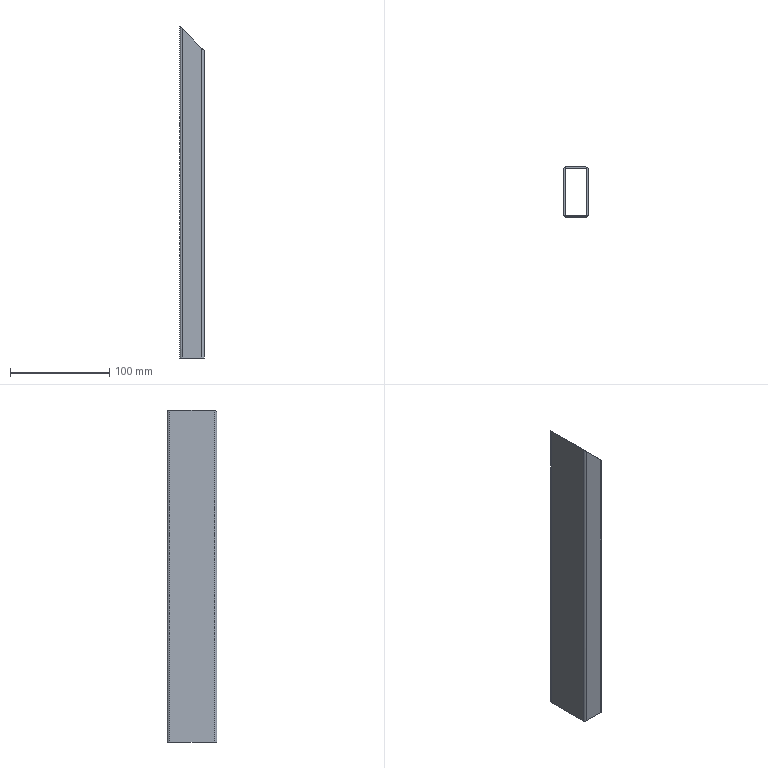Part | STEP file | 6150515 | 1 solid | 18 faces | box 25 x 50 x 334 mm | volume 67995 mm3 | plane 10 | cylinder 8 | commonest cylinder face diameters 2 x4 5 x4
STEP:
#1=CARTESIAN_POINT('',(-12.5,-22.5,0.));
#2=VERTEX_POINT('',#1);
#3=CARTESIAN_POINT('',(-10.,-25.,0.));
#4=VERTEX_POINT('',#3);
#5=CARTESIAN_POINT('',(-10.,-22.5,0.));
#6=DIRECTION('',(0.,0.,1.));
#7=DIRECTION('',(1.,0.,0.));
#8=AXIS2_PLACEMENT_3D('',#5,#6,#7);
#9=CIRCLE('',#8,2.5);
#10=EDGE_CURVE('',#2,#4,#9,.T.);
#11=ORIENTED_EDGE('',*,*,#10,.F.);
#12=CARTESIAN_POINT('',(-12.5,22.5,0.));
#13=VERTEX_POINT('',#12);
#14=CARTESIAN_POINT('',(-12.5,22.5,0.));
#15=DIRECTION('',(0.,-1.,0.));
#16=VECTOR('',#15,1000.);
#17=LINE('',#14,#16);
#18=EDGE_CURVE('',#13,#2,#17,.T.);
#19=ORIENTED_EDGE('',*,*,#18,.F.);
#20=CARTESIAN_POINT('',(-10.,25.,0.));
#21=VERTEX_POINT('',#20);
#22=CARTESIAN_POINT('',(-10.,22.5,0.));
#23=DIRECTION('',(0.,0.,1.));
#24=DIRECTION('',(1.,0.,0.));
#25=AXIS2_PLACEMENT_3D('',#22,#23,#24);
#26=CIRCLE('',#25,2.5);
#27=EDGE_CURVE('',#21,#13,#26,.T.);
#28=ORIENTED_EDGE('',*,*,#27,.F.);
#29=CARTESIAN_POINT('',(10.,25.,0.));
#30=VERTEX_POINT('',#29);
#31=CARTESIAN_POINT('',(-10.,25.,0.));
#32=DIRECTION('',(-1.,0.,0.));
#33=VECTOR('',#32,1000.);
#34=LINE('',#31,#33);
#35=EDGE_CURVE('',#30,#21,#34,.T.);
#36=ORIENTED_EDGE('',*,*,#35,.F.);
#37=CARTESIAN_POINT('',(12.5,22.5,0.));
#38=VERTEX_POINT('',#37);
#39=CARTESIAN_POINT('',(10.,22.5,0.));
#40=DIRECTION('',(0.,0.,1.));
#41=DIRECTION('',(-1.,0.,0.));
#42=AXIS2_PLACEMENT_3D('',#39,#40,#41);
#43=CIRCLE('',#42,2.5);
#44=EDGE_CURVE('',#38,#30,#43,.T.);
#45=ORIENTED_EDGE('',*,*,#44,.F.);
#46=CARTESIAN_POINT('',(12.5,-22.5,0.));
#47=VERTEX_POINT('',#46);
#48=CARTESIAN_POINT('',(12.5,22.5,0.));
#49=DIRECTION('',(0.,1.,0.));
#50=VECTOR('',#49,1000.);
#51=LINE('',#48,#50);
#52=EDGE_CURVE('',#47,#38,#51,.T.);
#53=ORIENTED_EDGE('',*,*,#52,.F.);
#54=CARTESIAN_POINT('',(10.,-25.,0.));
#55=VERTEX_POINT('',#54);
#56=CARTESIAN_POINT('',(10.,-22.5,0.));
#57=DIRECTION('',(0.,0.,1.));
#58=DIRECTION('',(1.,0.,0.));
#59=AXIS2_PLACEMENT_3D('',#56,#57,#58);
#60=CIRCLE('',#59,2.5);
#61=EDGE_CURVE('',#55,#47,#60,.T.);
#62=ORIENTED_EDGE('',*,*,#61,.F.);
#63=CARTESIAN_POINT('',(-10.,-25.,0.));
#64=DIRECTION('',(1.,0.,0.));
#65=VECTOR('',#64,1000.);
#66=LINE('',#63,#65);
#67=EDGE_CURVE('',#4,#55,#66,.T.);
#68=ORIENTED_EDGE('',*,*,#67,.F.);
#69=EDGE_LOOP('',(#11,#19,#28,#36,#45,#53,#62,#68));
#70=FACE_OUTER_BOUND('',#69,.T.);
#71=CARTESIAN_POINT('',(11.,22.5,0.));
#72=VERTEX_POINT('',#71);
#73=CARTESIAN_POINT('',(10.,23.5,0.));
#74=VERTEX_POINT('',#73);
#75=CARTESIAN_POINT('',(10.,22.5,0.));
#76=DIRECTION('',(0.,0.,1.));
#77=DIRECTION('',(-1.,0.,0.));
#78=AXIS2_PLACEMENT_3D('',#75,#76,#77);
#79=CIRCLE('',#78,1.);
#80=EDGE_CURVE('',#72,#74,#79,.T.);
#81=ORIENTED_EDGE('',*,*,#80,.T.);
#82=CARTESIAN_POINT('',(-10.,23.5,0.));
#83=VERTEX_POINT('',#82);
#84=CARTESIAN_POINT('',(-10.,23.5,0.));
#85=DIRECTION('',(-1.,0.,0.));
#86=VECTOR('',#85,1000.);
#87=LINE('',#84,#86);
#88=EDGE_CURVE('',#74,#83,#87,.T.);
#89=ORIENTED_EDGE('',*,*,#88,.T.);
#90=CARTESIAN_POINT('',(-11.,22.5,0.));
#91=VERTEX_POINT('',#90);
#92=CARTESIAN_POINT('',(-10.,22.5,0.));
#93=DIRECTION('',(0.,0.,1.));
#94=DIRECTION('',(1.,0.,0.));
#95=AXIS2_PLACEMENT_3D('',#92,#93,#94);
#96=CIRCLE('',#95,1.);
#97=EDGE_CURVE('',#83,#91,#96,.T.);
#98=ORIENTED_EDGE('',*,*,#97,.T.);
#99=CARTESIAN_POINT('',(-11.,-22.5,0.));
#100=VERTEX_POINT('',#99);
#101=CARTESIAN_POINT('',(-11.,22.5,0.));
#102=DIRECTION('',(0.,-1.,0.));
#103=VECTOR('',#102,1000.);
#104=LINE('',#101,#103);
#105=EDGE_CURVE('',#91,#100,#104,.T.);
#106=ORIENTED_EDGE('',*,*,#105,.T.);
#107=CARTESIAN_POINT('',(-10.,-23.5,0.));
#108=VERTEX_POINT('',#107);
#109=CARTESIAN_POINT('',(-10.,-22.5,0.));
#110=DIRECTION('',(0.,0.,1.));
#111=DIRECTION('',(1.,0.,0.));
#112=AXIS2_PLACEMENT_3D('',#109,#110,#111);
#113=CIRCLE('',#112,1.);
#114=EDGE_CURVE('',#100,#108,#113,.T.);
#115=ORIENTED_EDGE('',*,*,#114,.T.);
#116=CARTESIAN_POINT('',(10.,-23.5,0.));
#117=VERTEX_POINT('',#116);
#118=CARTESIAN_POINT('',(-10.,-23.5,0.));
#119=DIRECTION('',(1.,0.,0.));
#120=VECTOR('',#119,1000.);
#121=LINE('',#118,#120);
#122=EDGE_CURVE('',#108,#117,#121,.T.);
#123=ORIENTED_EDGE('',*,*,#122,.T.);
#124=CARTESIAN_POINT('',(11.,-22.5,0.));
#125=VERTEX_POINT('',#124);
#126=CARTESIAN_POINT('',(10.,-22.5,0.));
#127=DIRECTION('',(0.,0.,1.));
#128=DIRECTION('',(1.,0.,0.));
#129=AXIS2_PLACEMENT_3D('',#126,#127,#128);
#130=CIRCLE('',#129,1.);
#131=EDGE_CURVE('',#117,#125,#130,.T.);
#132=ORIENTED_EDGE('',*,*,#131,.T.);
#133=CARTESIAN_POINT('',(11.,22.5,0.));
#134=DIRECTION('',(0.,1.,0.));
#135=VECTOR('',#134,1000.);
#136=LINE('',#133,#135);
#137=EDGE_CURVE('',#125,#72,#136,.T.);
#138=ORIENTED_EDGE('',*,*,#137,.T.);
#139=EDGE_LOOP('',(#81,#89,#98,#106,#115,#123,#132,#138));
#140=FACE_BOUND('',#139,.T.);
#141=CARTESIAN_POINT('',(-10.,-22.5,0.));
#142=DIRECTION('',(0.,0.,1.));
#143=DIRECTION('',(1.,0.,0.));
#144=AXIS2_PLACEMENT_3D('',#141,#142,#143);
#145=PLANE('',#144);
#146=ADVANCED_FACE('',(#70,#140),#145,.F.);
#147=CARTESIAN_POINT('',(-10.,-25.,331.5));
#148=VERTEX_POINT('',#147);
#149=CARTESIAN_POINT('',(-10.,-25.,334.));
#150=DIRECTION('',(0.,0.,-1.));
#151=VECTOR('',#150,1000.);
#152=LINE('',#149,#151);
#153=EDGE_CURVE('',#148,#4,#152,.T.);
#154=ORIENTED_EDGE('',*,*,#153,.F.);
#155=CARTESIAN_POINT('',(-12.5,-22.5,334.));
#156=VERTEX_POINT('',#155);
#157=CARTESIAN_POINT('',(-10.,-25.,331.5));
#158=CARTESIAN_POINT('',(-11.464,-25.,332.964));
#159=CARTESIAN_POINT('',(-12.5,-23.964,334.));
#160=CARTESIAN_POINT('',(-12.5,-22.5,334.));
#161=(BOUNDED_CURVE()B_SPLINE_CURVE(3,(#157,#158,#159,#160),.UNSPECIFIED.,.F.,.F.)B_SPLINE_CURVE_WITH_KNOTS((4,4),(1.571,3.142),.UNSPECIFIED.)CURVE()GEOMETRIC_REPRESENTATION_ITEM()RATIONAL_B_SPLINE_CURVE((1.,0.8047,0.8047,1.))REPRESENTATION_ITEM(''));
#162=EDGE_CURVE('',#148,#156,#161,.T.);
#163=ORIENTED_EDGE('',*,*,#162,.T.);
#164=CARTESIAN_POINT('',(-12.5,-22.5,334.));
#165=DIRECTION('',(0.,0.,-1.));
#166=VECTOR('',#165,1000.);
#167=LINE('',#164,#166);
#168=EDGE_CURVE('',#156,#2,#167,.T.);
#169=ORIENTED_EDGE('',*,*,#168,.T.);
#170=ORIENTED_EDGE('',*,*,#10,.T.);
#171=EDGE_LOOP('',(#154,#163,#169,#170));
#172=FACE_OUTER_BOUND('',#171,.T.);
#173=CARTESIAN_POINT('',(-10.,-22.5,334.));
#174=DIRECTION('',(0.,0.,-1.));
#175=DIRECTION('',(-1.,0.,0.));
#176=AXIS2_PLACEMENT_3D('',#173,#174,#175);
#177=CYLINDRICAL_SURFACE('',#176,2.5);
#178=ADVANCED_FACE('',(#172),#177,.T.);
#179=CARTESIAN_POINT('',(10.,-25.,311.5));
#180=VERTEX_POINT('',#179);
#181=CARTESIAN_POINT('',(10.,-25.,334.));
#182=DIRECTION('',(0.,0.,-1.));
#183=VECTOR('',#182,1000.);
#184=LINE('',#181,#183);
#185=EDGE_CURVE('',#180,#55,#184,.T.);
#186=ORIENTED_EDGE('',*,*,#185,.F.);
#187=CARTESIAN_POINT('',(-11.25,-25.,332.75));
#188=DIRECTION('',(-0.7071,0.,0.7071));
#189=VECTOR('',#188,1000.);
#190=LINE('',#187,#189);
#191=EDGE_CURVE('',#180,#148,#190,.T.);
#192=ORIENTED_EDGE('',*,*,#191,.T.);
#193=ORIENTED_EDGE('',*,*,#153,.T.);
#194=ORIENTED_EDGE('',*,*,#67,.T.);
#195=EDGE_LOOP('',(#186,#192,#193,#194));
#196=FACE_OUTER_BOUND('',#195,.T.);
#197=CARTESIAN_POINT('',(-10.,-25.,334.));
#198=DIRECTION('',(0.,1.,0.));
#199=DIRECTION('',(-1.,0.,0.));
#200=AXIS2_PLACEMENT_3D('',#197,#198,#199);
#201=PLANE('',#200);
#202=ADVANCED_FACE('',(#196),#201,.F.);
#203=CARTESIAN_POINT('',(12.5,-22.5,309.));
#204=VERTEX_POINT('',#203);
#205=CARTESIAN_POINT('',(12.5,-22.5,334.));
#206=DIRECTION('',(0.,0.,-1.));
#207=VECTOR('',#206,1000.);
#208=LINE('',#205,#207);
#209=EDGE_CURVE('',#204,#47,#208,.T.);
#210=ORIENTED_EDGE('',*,*,#209,.F.);
#211=CARTESIAN_POINT('',(12.5,-22.5,309.));
#212=CARTESIAN_POINT('',(12.5,-23.964,309.));
#213=CARTESIAN_POINT('',(11.464,-25.,310.036));
#214=CARTESIAN_POINT('',(10.,-25.,311.5));
#215=(BOUNDED_CURVE()B_SPLINE_CURVE(3,(#211,#212,#213,#214),.UNSPECIFIED.,.F.,.F.)B_SPLINE_CURVE_WITH_KNOTS((4,4),(0.,1.571),.UNSPECIFIED.)CURVE()GEOMETRIC_REPRESENTATION_ITEM()RATIONAL_B_SPLINE_CURVE((1.,0.8047,0.8047,1.))REPRESENTATION_ITEM(''));
#216=EDGE_CURVE('',#204,#180,#215,.T.);
#217=ORIENTED_EDGE('',*,*,#216,.T.);
#218=ORIENTED_EDGE('',*,*,#185,.T.);
#219=ORIENTED_EDGE('',*,*,#61,.T.);
#220=EDGE_LOOP('',(#210,#217,#218,#219));
#221=FACE_OUTER_BOUND('',#220,.T.);
#222=CARTESIAN_POINT('',(10.,-22.5,334.));
#223=DIRECTION('',(0.,0.,-1.));
#224=DIRECTION('',(-1.,0.,0.));
#225=AXIS2_PLACEMENT_3D('',#222,#223,#224);
#226=CYLINDRICAL_SURFACE('',#225,2.5);
#227=ADVANCED_FACE('',(#221),#226,.T.);
#228=CARTESIAN_POINT('',(12.5,22.5,309.));
#229=VERTEX_POINT('',#228);
#230=CARTESIAN_POINT('',(12.5,22.5,334.));
#231=DIRECTION('',(0.,0.,-1.));
#232=VECTOR('',#231,1000.);
#233=LINE('',#230,#232);
#234=EDGE_CURVE('',#229,#38,#233,.T.);
#235=ORIENTED_EDGE('',*,*,#234,.F.);
#236=CARTESIAN_POINT('',(12.5,22.5,309.));
#237=DIRECTION('',(0.,-1.,0.));
#238=VECTOR('',#237,1000.);
#239=LINE('',#236,#238);
#240=EDGE_CURVE('',#229,#204,#239,.T.);
#241=ORIENTED_EDGE('',*,*,#240,.T.);
#242=ORIENTED_EDGE('',*,*,#209,.T.);
#243=ORIENTED_EDGE('',*,*,#52,.T.);
#244=EDGE_LOOP('',(#235,#241,#242,#243));
#245=FACE_OUTER_BOUND('',#244,.T.);
#246=CARTESIAN_POINT('',(12.5,22.5,334.));
#247=DIRECTION('',(-1.,0.,0.));
#248=DIRECTION('',(0.,-1.,0.));
#249=AXIS2_PLACEMENT_3D('',#246,#247,#248);
#250=PLANE('',#249);
#251=ADVANCED_FACE('',(#245),#250,.F.);
#252=CARTESIAN_POINT('',(10.,25.,311.5));
#253=VERTEX_POINT('',#252);
#254=CARTESIAN_POINT('',(10.,25.,334.));
#255=DIRECTION('',(0.,0.,-1.));
#256=VECTOR('',#255,1000.);
#257=LINE('',#254,#256);
#258=EDGE_CURVE('',#253,#30,#257,.T.);
#259=ORIENTED_EDGE('',*,*,#258,.F.);
#260=CARTESIAN_POINT('',(10.,25.,311.5));
#261=CARTESIAN_POINT('',(11.464,25.,310.036));
#262=CARTESIAN_POINT('',(12.5,23.964,309.));
#263=CARTESIAN_POINT('',(12.5,22.5,309.));
#264=(BOUNDED_CURVE()B_SPLINE_CURVE(3,(#260,#261,#262,#263),.UNSPECIFIED.,.F.,.F.)B_SPLINE_CURVE_WITH_KNOTS((4,4),(4.712,6.283),.UNSPECIFIED.)CURVE()GEOMETRIC_REPRESENTATION_ITEM()RATIONAL_B_SPLINE_CURVE((1.,0.8047,0.8047,1.))REPRESENTATION_ITEM(''));
#265=EDGE_CURVE('',#253,#229,#264,.T.);
#266=ORIENTED_EDGE('',*,*,#265,.T.);
#267=ORIENTED_EDGE('',*,*,#234,.T.);
#268=ORIENTED_EDGE('',*,*,#44,.T.);
#269=EDGE_LOOP('',(#259,#266,#267,#268));
#270=FACE_OUTER_BOUND('',#269,.T.);
#271=CARTESIAN_POINT('',(10.,22.5,334.));
#272=DIRECTION('',(0.,0.,-1.));
#273=DIRECTION('',(-1.,0.,0.));
#274=AXIS2_PLACEMENT_3D('',#271,#272,#273);
#275=CYLINDRICAL_SURFACE('',#274,2.5);
#276=ADVANCED_FACE('',(#270),#275,.T.);
#277=CARTESIAN_POINT('',(-10.,25.,331.5));
#278=VERTEX_POINT('',#277);
#279=CARTESIAN_POINT('',(-10.,25.,334.));
#280=DIRECTION('',(0.,0.,-1.));
#281=VECTOR('',#280,1000.);
#282=LINE('',#279,#281);
#283=EDGE_CURVE('',#278,#21,#282,.T.);
#284=ORIENTED_EDGE('',*,*,#283,.F.);
#285=CARTESIAN_POINT('',(-11.25,25.,332.75));
#286=DIRECTION('',(0.7071,0.,-0.7071));
#287=VECTOR('',#286,1000.);
#288=LINE('',#285,#287);
#289=EDGE_CURVE('',#278,#253,#288,.T.);
#290=ORIENTED_EDGE('',*,*,#289,.T.);
#291=ORIENTED_EDGE('',*,*,#258,.T.);
#292=ORIENTED_EDGE('',*,*,#35,.T.);
#293=EDGE_LOOP('',(#284,#290,#291,#292));
#294=FACE_OUTER_BOUND('',#293,.T.);
#295=CARTESIAN_POINT('',(-10.,25.,334.));
#296=DIRECTION('',(0.,-1.,0.));
#297=DIRECTION('',(0.,0.,-1.));
#298=AXIS2_PLACEMENT_3D('',#295,#296,#297);
#299=PLANE('',#298);
#300=ADVANCED_FACE('',(#294),#299,.F.);
#301=CARTESIAN_POINT('',(-12.5,22.5,334.));
#302=VERTEX_POINT('',#301);
#303=CARTESIAN_POINT('',(-12.5,22.5,334.));
#304=DIRECTION('',(0.,0.,-1.));
#305=VECTOR('',#304,1000.);
#306=LINE('',#303,#305);
#307=EDGE_CURVE('',#302,#13,#306,.T.);
#308=ORIENTED_EDGE('',*,*,#307,.F.);
#309=CARTESIAN_POINT('',(-12.5,22.5,334.));
#310=CARTESIAN_POINT('',(-12.5,23.964,334.));
#311=CARTESIAN_POINT('',(-11.464,25.,332.964));
#312=CARTESIAN_POINT('',(-10.,25.,331.5));
#313=(BOUNDED_CURVE()B_SPLINE_CURVE(3,(#309,#310,#311,#312),.UNSPECIFIED.,.F.,.F.)B_SPLINE_CURVE_WITH_KNOTS((4,4),(3.142,4.712),.UNSPECIFIED.)CURVE()GEOMETRIC_REPRESENTATION_ITEM()RATIONAL_B_SPLINE_CURVE((1.,0.8047,0.8047,1.))REPRESENTATION_ITEM(''));
#314=EDGE_CURVE('',#302,#278,#313,.T.);
#315=ORIENTED_EDGE('',*,*,#314,.T.);
#316=ORIENTED_EDGE('',*,*,#283,.T.);
#317=ORIENTED_EDGE('',*,*,#27,.T.);
#318=EDGE_LOOP('',(#308,#315,#316,#317));
#319=FACE_OUTER_BOUND('',#318,.T.);
#320=CARTESIAN_POINT('',(-10.,22.5,334.));
#321=DIRECTION('',(0.,0.,-1.));
#322=DIRECTION('',(-1.,0.,0.));
#323=AXIS2_PLACEMENT_3D('',#320,#321,#322);
#324=CYLINDRICAL_SURFACE('',#323,2.5);
#325=ADVANCED_FACE('',(#319),#324,.T.);
#326=ORIENTED_EDGE('',*,*,#18,.T.);
#327=ORIENTED_EDGE('',*,*,#168,.F.);
#328=CARTESIAN_POINT('',(-12.5,22.5,334.));
#329=DIRECTION('',(0.,-1.,0.));
#330=VECTOR('',#329,1000.);
#331=LINE('',#328,#330);
#332=EDGE_CURVE('',#302,#156,#331,.T.);
#333=ORIENTED_EDGE('',*,*,#332,.F.);
#334=ORIENTED_EDGE('',*,*,#307,.T.);
#335=EDGE_LOOP('',(#326,#327,#333,#334));
#336=FACE_OUTER_BOUND('',#335,.T.);
#337=CARTESIAN_POINT('',(-12.5,22.5,334.));
#338=DIRECTION('',(1.,0.,0.));
#339=DIRECTION('',(0.,1.,0.));
#340=AXIS2_PLACEMENT_3D('',#337,#338,#339);
#341=PLANE('',#340);
#342=ADVANCED_FACE('',(#336),#341,.F.);
#343=CARTESIAN_POINT('',(10.,23.5,311.5));
#344=VERTEX_POINT('',#343);
#345=CARTESIAN_POINT('',(11.,22.5,310.5));
#346=VERTEX_POINT('',#345);
#347=CARTESIAN_POINT('',(10.,23.5,311.5));
#348=CARTESIAN_POINT('',(10.586,23.5,310.914));
#349=CARTESIAN_POINT('',(11.,23.086,310.5));
#350=CARTESIAN_POINT('',(11.,22.5,310.5));
#351=(BOUNDED_CURVE()B_SPLINE_CURVE(3,(#347,#348,#349,#350),.UNSPECIFIED.,.F.,.F.)B_SPLINE_CURVE_WITH_KNOTS((4,4),(4.712,6.283),.UNSPECIFIED.)CURVE()GEOMETRIC_REPRESENTATION_ITEM()RATIONAL_B_SPLINE_CURVE((1.,0.8047,0.8047,1.))REPRESENTATION_ITEM(''));
#352=EDGE_CURVE('',#344,#346,#351,.T.);
#353=ORIENTED_EDGE('',*,*,#352,.F.);
#354=CARTESIAN_POINT('',(10.,23.5,334.));
#355=DIRECTION('',(0.,0.,-1.));
#356=VECTOR('',#355,1000.);
#357=LINE('',#354,#356);
#358=EDGE_CURVE('',#344,#74,#357,.T.);
#359=ORIENTED_EDGE('',*,*,#358,.T.);
#360=ORIENTED_EDGE('',*,*,#80,.F.);
#361=CARTESIAN_POINT('',(11.,22.5,334.));
#362=DIRECTION('',(0.,0.,-1.));
#363=VECTOR('',#362,1000.);
#364=LINE('',#361,#363);
#365=EDGE_CURVE('',#346,#72,#364,.T.);
#366=ORIENTED_EDGE('',*,*,#365,.F.);
#367=EDGE_LOOP('',(#353,#359,#360,#366));
#368=FACE_OUTER_BOUND('',#367,.T.);
#369=CARTESIAN_POINT('',(10.,22.5,334.));
#370=DIRECTION('',(0.,0.,-1.));
#371=DIRECTION('',(-1.,0.,0.));
#372=AXIS2_PLACEMENT_3D('',#369,#370,#371);
#373=CYLINDRICAL_SURFACE('',#372,1.);
#374=ADVANCED_FACE('',(#368),#373,.F.);
#375=CARTESIAN_POINT('',(-10.,23.5,331.5));
#376=VERTEX_POINT('',#375);
#377=CARTESIAN_POINT('',(-11.25,23.5,332.75));
#378=DIRECTION('',(0.7071,0.,-0.7071));
#379=VECTOR('',#378,1000.);
#380=LINE('',#377,#379);
#381=EDGE_CURVE('',#376,#344,#380,.T.);
#382=ORIENTED_EDGE('',*,*,#381,.F.);
#383=CARTESIAN_POINT('',(-10.,23.5,334.));
#384=DIRECTION('',(0.,0.,-1.));
#385=VECTOR('',#384,1000.);
#386=LINE('',#383,#385);
#387=EDGE_CURVE('',#376,#83,#386,.T.);
#388=ORIENTED_EDGE('',*,*,#387,.T.);
#389=ORIENTED_EDGE('',*,*,#88,.F.);
#390=ORIENTED_EDGE('',*,*,#358,.F.);
#391=EDGE_LOOP('',(#382,#388,#389,#390));
#392=FACE_OUTER_BOUND('',#391,.T.);
#393=CARTESIAN_POINT('',(-10.,23.5,334.));
#394=DIRECTION('',(0.,-1.,0.));
#395=DIRECTION('',(1.,0.,0.));
#396=AXIS2_PLACEMENT_3D('',#393,#394,#395);
#397=PLANE('',#396);
#398=ADVANCED_FACE('',(#392),#397,.T.);
#399=CARTESIAN_POINT('',(-11.,22.5,332.5));
#400=VERTEX_POINT('',#399);
#401=CARTESIAN_POINT('',(-11.,22.5,332.5));
#402=CARTESIAN_POINT('',(-11.,23.086,332.5));
#403=CARTESIAN_POINT('',(-10.586,23.5,332.086));
#404=CARTESIAN_POINT('',(-10.,23.5,331.5));
#405=(BOUNDED_CURVE()B_SPLINE_CURVE(3,(#401,#402,#403,#404),.UNSPECIFIED.,.F.,.F.)B_SPLINE_CURVE_WITH_KNOTS((4,4),(3.142,4.712),.UNSPECIFIED.)CURVE()GEOMETRIC_REPRESENTATION_ITEM()RATIONAL_B_SPLINE_CURVE((1.,0.8047,0.8047,1.))REPRESENTATION_ITEM(''));
#406=EDGE_CURVE('',#400,#376,#405,.T.);
#407=ORIENTED_EDGE('',*,*,#406,.F.);
#408=CARTESIAN_POINT('',(-11.,22.5,334.));
#409=DIRECTION('',(0.,0.,-1.));
#410=VECTOR('',#409,1000.);
#411=LINE('',#408,#410);
#412=EDGE_CURVE('',#400,#91,#411,.T.);
#413=ORIENTED_EDGE('',*,*,#412,.T.);
#414=ORIENTED_EDGE('',*,*,#97,.F.);
#415=ORIENTED_EDGE('',*,*,#387,.F.);
#416=EDGE_LOOP('',(#407,#413,#414,#415));
#417=FACE_OUTER_BOUND('',#416,.T.);
#418=CARTESIAN_POINT('',(-10.,22.5,334.));
#419=DIRECTION('',(0.,0.,-1.));
#420=DIRECTION('',(-1.,0.,0.));
#421=AXIS2_PLACEMENT_3D('',#418,#419,#420);
#422=CYLINDRICAL_SURFACE('',#421,1.);
#423=ADVANCED_FACE('',(#417),#422,.F.);
#424=CARTESIAN_POINT('',(-11.,-22.5,332.5));
#425=VERTEX_POINT('',#424);
#426=CARTESIAN_POINT('',(-11.,22.5,332.5));
#427=DIRECTION('',(0.,1.,0.));
#428=VECTOR('',#427,1000.);
#429=LINE('',#426,#428);
#430=EDGE_CURVE('',#425,#400,#429,.T.);
#431=ORIENTED_EDGE('',*,*,#430,.F.);
#432=CARTESIAN_POINT('',(-11.,-22.5,334.));
#433=DIRECTION('',(0.,0.,-1.));
#434=VECTOR('',#433,1000.);
#435=LINE('',#432,#434);
#436=EDGE_CURVE('',#425,#100,#435,.T.);
#437=ORIENTED_EDGE('',*,*,#436,.T.);
#438=ORIENTED_EDGE('',*,*,#105,.F.);
#439=ORIENTED_EDGE('',*,*,#412,.F.);
#440=EDGE_LOOP('',(#431,#437,#438,#439));
#441=FACE_OUTER_BOUND('',#440,.T.);
#442=CARTESIAN_POINT('',(-11.,22.5,334.));
#443=DIRECTION('',(1.,0.,0.));
#444=DIRECTION('',(0.,1.,0.));
#445=AXIS2_PLACEMENT_3D('',#442,#443,#444);
#446=PLANE('',#445);
#447=ADVANCED_FACE('',(#441),#446,.T.);
#448=CARTESIAN_POINT('',(-10.,-23.5,331.5));
#449=VERTEX_POINT('',#448);
#450=CARTESIAN_POINT('',(-10.,-23.5,331.5));
#451=CARTESIAN_POINT('',(-10.586,-23.5,332.086));
#452=CARTESIAN_POINT('',(-11.,-23.086,332.5));
#453=CARTESIAN_POINT('',(-11.,-22.5,332.5));
#454=(BOUNDED_CURVE()B_SPLINE_CURVE(3,(#450,#451,#452,#453),.UNSPECIFIED.,.F.,.T.)B_SPLINE_CURVE_WITH_KNOTS((4,4),(1.571,3.142),.UNSPECIFIED.)CURVE()GEOMETRIC_REPRESENTATION_ITEM()RATIONAL_B_SPLINE_CURVE((1.,0.8047,0.8047,1.))REPRESENTATION_ITEM(''));
#455=EDGE_CURVE('',#449,#425,#454,.T.);
#456=ORIENTED_EDGE('',*,*,#455,.F.);
#457=CARTESIAN_POINT('',(-10.,-23.5,334.));
#458=DIRECTION('',(0.,0.,-1.));
#459=VECTOR('',#458,1000.);
#460=LINE('',#457,#459);
#461=EDGE_CURVE('',#449,#108,#460,.T.);
#462=ORIENTED_EDGE('',*,*,#461,.T.);
#463=ORIENTED_EDGE('',*,*,#114,.F.);
#464=ORIENTED_EDGE('',*,*,#436,.F.);
#465=EDGE_LOOP('',(#456,#462,#463,#464));
#466=FACE_OUTER_BOUND('',#465,.T.);
#467=CARTESIAN_POINT('',(-10.,-22.5,334.));
#468=DIRECTION('',(0.,0.,-1.));
#469=DIRECTION('',(-1.,0.,0.));
#470=AXIS2_PLACEMENT_3D('',#467,#468,#469);
#471=CYLINDRICAL_SURFACE('',#470,1.);
#472=ADVANCED_FACE('',(#466),#471,.F.);
#473=CARTESIAN_POINT('',(10.,-23.5,311.5));
#474=VERTEX_POINT('',#473);
#475=CARTESIAN_POINT('',(-11.25,-23.5,332.75));
#476=DIRECTION('',(-0.7071,0.,0.7071));
#477=VECTOR('',#476,1000.);
#478=LINE('',#475,#477);
#479=EDGE_CURVE('',#474,#449,#478,.T.);
#480=ORIENTED_EDGE('',*,*,#479,.F.);
#481=CARTESIAN_POINT('',(10.,-23.5,334.));
#482=DIRECTION('',(0.,0.,-1.));
#483=VECTOR('',#482,1000.);
#484=LINE('',#481,#483);
#485=EDGE_CURVE('',#474,#117,#484,.T.);
#486=ORIENTED_EDGE('',*,*,#485,.T.);
#487=ORIENTED_EDGE('',*,*,#122,.F.);
#488=ORIENTED_EDGE('',*,*,#461,.F.);
#489=EDGE_LOOP('',(#480,#486,#487,#488));
#490=FACE_OUTER_BOUND('',#489,.T.);
#491=CARTESIAN_POINT('',(-10.,-23.5,334.));
#492=DIRECTION('',(0.,1.,0.));
#493=DIRECTION('',(-1.,0.,0.));
#494=AXIS2_PLACEMENT_3D('',#491,#492,#493);
#495=PLANE('',#494);
#496=ADVANCED_FACE('',(#490),#495,.T.);
#497=CARTESIAN_POINT('',(11.,-22.5,310.5));
#498=VERTEX_POINT('',#497);
#499=CARTESIAN_POINT('',(11.,-22.5,310.5));
#500=CARTESIAN_POINT('',(11.,-23.086,310.5));
#501=CARTESIAN_POINT('',(10.586,-23.5,310.914));
#502=CARTESIAN_POINT('',(10.,-23.5,311.5));
#503=(BOUNDED_CURVE()B_SPLINE_CURVE(3,(#499,#500,#501,#502),.UNSPECIFIED.,.F.,.F.)B_SPLINE_CURVE_WITH_KNOTS((4,4),(0.,1.571),.UNSPECIFIED.)CURVE()GEOMETRIC_REPRESENTATION_ITEM()RATIONAL_B_SPLINE_CURVE((1.,0.8047,0.8047,1.))REPRESENTATION_ITEM(''));
#504=EDGE_CURVE('',#498,#474,#503,.T.);
#505=ORIENTED_EDGE('',*,*,#504,.F.);
#506=CARTESIAN_POINT('',(11.,-22.5,334.));
#507=DIRECTION('',(0.,0.,-1.));
#508=VECTOR('',#507,1000.);
#509=LINE('',#506,#508);
#510=EDGE_CURVE('',#498,#125,#509,.T.);
#511=ORIENTED_EDGE('',*,*,#510,.T.);
#512=ORIENTED_EDGE('',*,*,#131,.F.);
#513=ORIENTED_EDGE('',*,*,#485,.F.);
#514=EDGE_LOOP('',(#505,#511,#512,#513));
#515=FACE_OUTER_BOUND('',#514,.T.);
#516=CARTESIAN_POINT('',(10.,-22.5,334.));
#517=DIRECTION('',(0.,0.,-1.));
#518=DIRECTION('',(-1.,0.,0.));
#519=AXIS2_PLACEMENT_3D('',#516,#517,#518);
#520=CYLINDRICAL_SURFACE('',#519,1.);
#521=ADVANCED_FACE('',(#515),#520,.F.);
#522=CARTESIAN_POINT('',(11.,22.5,310.5));
#523=DIRECTION('',(0.,-1.,0.));
#524=VECTOR('',#523,1000.);
#525=LINE('',#522,#524);
#526=EDGE_CURVE('',#346,#498,#525,.T.);
#527=ORIENTED_EDGE('',*,*,#526,.F.);
#528=ORIENTED_EDGE('',*,*,#365,.T.);
#529=ORIENTED_EDGE('',*,*,#137,.F.);
#530=ORIENTED_EDGE('',*,*,#510,.F.);
#531=EDGE_LOOP('',(#527,#528,#529,#530));
#532=FACE_OUTER_BOUND('',#531,.T.);
#533=CARTESIAN_POINT('',(11.,22.5,334.));
#534=DIRECTION('',(-1.,0.,0.));
#535=DIRECTION('',(0.,0.,1.));
#536=AXIS2_PLACEMENT_3D('',#533,#534,#535);
#537=PLANE('',#536);
#538=ADVANCED_FACE('',(#532),#537,.T.);
#539=ORIENTED_EDGE('',*,*,#381,.T.);
#540=ORIENTED_EDGE('',*,*,#352,.T.);
#541=ORIENTED_EDGE('',*,*,#526,.T.);
#542=ORIENTED_EDGE('',*,*,#504,.T.);
#543=ORIENTED_EDGE('',*,*,#479,.T.);
#544=ORIENTED_EDGE('',*,*,#455,.T.);
#545=ORIENTED_EDGE('',*,*,#430,.T.);
#546=ORIENTED_EDGE('',*,*,#406,.T.);
#547=EDGE_LOOP('',(#539,#540,#541,#542,#543,#544,#545,#546));
#548=FACE_BOUND('',#547,.T.);
#549=ORIENTED_EDGE('',*,*,#162,.F.);
#550=ORIENTED_EDGE('',*,*,#191,.F.);
#551=ORIENTED_EDGE('',*,*,#216,.F.);
#552=ORIENTED_EDGE('',*,*,#240,.F.);
#553=ORIENTED_EDGE('',*,*,#265,.F.);
#554=ORIENTED_EDGE('',*,*,#289,.F.);
#555=ORIENTED_EDGE('',*,*,#314,.F.);
#556=ORIENTED_EDGE('',*,*,#332,.T.);
#557=EDGE_LOOP('',(#549,#550,#551,#552,#553,#554,#555,#556));
#558=FACE_OUTER_BOUND('',#557,.T.);
#559=CARTESIAN_POINT('',(-12.5,510.807,334.));
#560=DIRECTION('',(-0.7071,0.,-0.7071));
#561=DIRECTION('',(-0.7071,0.,0.7071));
#562=AXIS2_PLACEMENT_3D('',#559,#560,#561);
#563=PLANE('',#562);
#564=ADVANCED_FACE('',(#548,#558),#563,.F.);
#565=CLOSED_SHELL('',(#146,#178,#202,#227,#251,#276,#300,#325,#342,#374,#398,#423,#447,#472,#496,#521,#538,#564));
#566=MANIFOLD_SOLID_BREP('',#565);
#567=CARTESIAN_POINT('',(0.,0.,0.));
#568=DIRECTION('',(0.,0.,1.));
#569=DIRECTION('',(1.,0.,0.));
#570=AXIS2_PLACEMENT_3D('',#567,#568,#569);
#571=(LENGTH_UNIT()NAMED_UNIT(*)SI_UNIT(.MILLI.,.METRE.));
#572=UNCERTAINTY_MEASURE_WITH_UNIT(LENGTH_MEASURE(0.00001),#571,'','');
#573=(NAMED_UNIT(*)PLANE_ANGLE_UNIT()SI_UNIT($,.RADIAN.));
#574=(NAMED_UNIT(*)SI_UNIT($,.STERADIAN.)SOLID_ANGLE_UNIT());
#575=(GEOMETRIC_REPRESENTATION_CONTEXT(3)GLOBAL_UNCERTAINTY_ASSIGNED_CONTEXT((#572))GLOBAL_UNIT_ASSIGNED_CONTEXT((#571,#573,#574))REPRESENTATION_CONTEXT('',''));
#576=ADVANCED_BREP_SHAPE_REPRESENTATION('',(#566,#570),#575);